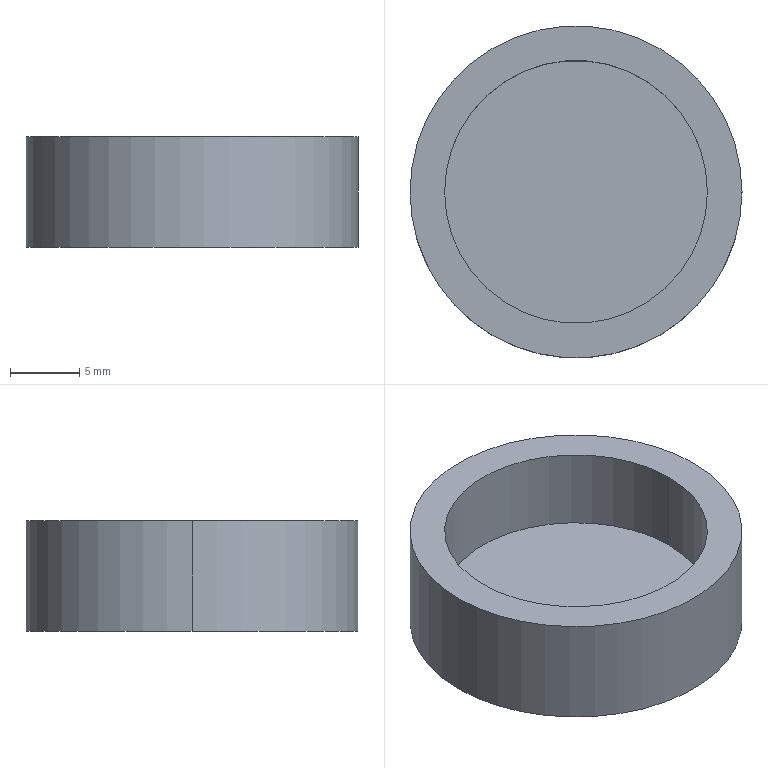Part | SolidWorks | features Extrusion 1, ICE 1 | 1 solid | 7 faces | box 24 x 24 x 8 mm | volume 1918 mm3 | cylinder 4 | plane 3 | commonest cylinder face diameters 19 x2 24 x2
STEP:
#1=CARTESIAN_POINT('',(-9.5,0.,2.));
#2=VERTEX_POINT('',#1);
#3=CARTESIAN_POINT('',(9.5,0.,2.));
#4=VERTEX_POINT('',#3);
#5=CARTESIAN_POINT('',(0.,0.,2.));
#6=DIRECTION('',(0.,0.,1.));
#7=DIRECTION('',(1.,0.,0.));
#8=AXIS2_PLACEMENT_3D('',#5,#6,#7);
#9=CIRCLE('',#8,9.5);
#10=EDGE_CURVE('',#2,#4,#9,.T.);
#11=ORIENTED_EDGE('',*,*,#10,.F.);
#12=CARTESIAN_POINT('',(-9.5,0.,8.));
#13=VERTEX_POINT('',#12);
#14=CARTESIAN_POINT('',(-9.5,0.,2.));
#15=DIRECTION('',(0.,0.,1.));
#16=VECTOR('',#15,1000.);
#17=LINE('',#14,#16);
#18=EDGE_CURVE('',#2,#13,#17,.T.);
#19=ORIENTED_EDGE('',*,*,#18,.T.);
#20=CARTESIAN_POINT('',(9.5,0.,8.));
#21=VERTEX_POINT('',#20);
#22=CARTESIAN_POINT('',(0.,0.,8.));
#23=DIRECTION('',(0.,0.,1.));
#24=DIRECTION('',(1.,0.,0.));
#25=AXIS2_PLACEMENT_3D('',#22,#23,#24);
#26=CIRCLE('',#25,9.5);
#27=EDGE_CURVE('',#13,#21,#26,.T.);
#28=ORIENTED_EDGE('',*,*,#27,.T.);
#29=CARTESIAN_POINT('',(9.5,0.,2.));
#30=DIRECTION('',(0.,0.,1.));
#31=VECTOR('',#30,1000.);
#32=LINE('',#29,#31);
#33=EDGE_CURVE('',#4,#21,#32,.T.);
#34=ORIENTED_EDGE('',*,*,#33,.F.);
#35=EDGE_LOOP('',(#11,#19,#28,#34));
#36=FACE_OUTER_BOUND('',#35,.T.);
#37=CARTESIAN_POINT('',(0.,0.,2.));
#38=DIRECTION('',(0.,0.,1.));
#39=DIRECTION('',(1.,0.,0.));
#40=AXIS2_PLACEMENT_3D('',#37,#38,#39);
#41=CYLINDRICAL_SURFACE('',#40,9.5);
#42=ADVANCED_FACE('',(#36),#41,.F.);
#43=CARTESIAN_POINT('',(12.,0.,8.));
#44=VERTEX_POINT('',#43);
#45=CARTESIAN_POINT('',(-12.,0.,8.));
#46=VERTEX_POINT('',#45);
#47=CARTESIAN_POINT('',(0.,0.,8.));
#48=DIRECTION('',(0.,0.,1.));
#49=DIRECTION('',(1.,0.,0.));
#50=AXIS2_PLACEMENT_3D('',#47,#48,#49);
#51=CIRCLE('',#50,12.);
#52=EDGE_CURVE('',#44,#46,#51,.T.);
#53=ORIENTED_EDGE('',*,*,#52,.F.);
#54=CARTESIAN_POINT('',(12.,0.,0.));
#55=VERTEX_POINT('',#54);
#56=CARTESIAN_POINT('',(12.,0.,8.));
#57=DIRECTION('',(0.,0.,-1.));
#58=VECTOR('',#57,1000.);
#59=LINE('',#56,#58);
#60=EDGE_CURVE('',#44,#55,#59,.T.);
#61=ORIENTED_EDGE('',*,*,#60,.T.);
#62=CARTESIAN_POINT('',(-12.,0.,0.));
#63=VERTEX_POINT('',#62);
#64=CARTESIAN_POINT('',(0.,0.,0.));
#65=DIRECTION('',(0.,0.,1.));
#66=DIRECTION('',(1.,0.,0.));
#67=AXIS2_PLACEMENT_3D('',#64,#65,#66);
#68=CIRCLE('',#67,12.);
#69=EDGE_CURVE('',#55,#63,#68,.T.);
#70=ORIENTED_EDGE('',*,*,#69,.T.);
#71=CARTESIAN_POINT('',(-12.,0.,8.));
#72=DIRECTION('',(0.,0.,-1.));
#73=VECTOR('',#72,1000.);
#74=LINE('',#71,#73);
#75=EDGE_CURVE('',#46,#63,#74,.T.);
#76=ORIENTED_EDGE('',*,*,#75,.F.);
#77=EDGE_LOOP('',(#53,#61,#70,#76));
#78=FACE_OUTER_BOUND('',#77,.T.);
#79=CARTESIAN_POINT('',(0.,0.,8.));
#80=DIRECTION('',(0.,0.,-1.));
#81=DIRECTION('',(-1.,0.,0.));
#82=AXIS2_PLACEMENT_3D('',#79,#80,#81);
#83=CYLINDRICAL_SURFACE('',#82,12.);
#84=ADVANCED_FACE('',(#78),#83,.T.);
#85=ORIENTED_EDGE('',*,*,#60,.F.);
#86=CARTESIAN_POINT('',(0.,0.,8.));
#87=DIRECTION('',(0.,0.,1.));
#88=DIRECTION('',(1.,0.,0.));
#89=AXIS2_PLACEMENT_3D('',#86,#87,#88);
#90=CIRCLE('',#89,12.);
#91=EDGE_CURVE('',#46,#44,#90,.T.);
#92=ORIENTED_EDGE('',*,*,#91,.F.);
#93=ORIENTED_EDGE('',*,*,#75,.T.);
#94=CARTESIAN_POINT('',(0.,0.,0.));
#95=DIRECTION('',(0.,0.,1.));
#96=DIRECTION('',(1.,0.,0.));
#97=AXIS2_PLACEMENT_3D('',#94,#95,#96);
#98=CIRCLE('',#97,12.);
#99=EDGE_CURVE('',#63,#55,#98,.T.);
#100=ORIENTED_EDGE('',*,*,#99,.T.);
#101=EDGE_LOOP('',(#85,#92,#93,#100));
#102=FACE_OUTER_BOUND('',#101,.T.);
#103=CARTESIAN_POINT('',(0.,0.,8.));
#104=DIRECTION('',(0.,0.,-1.));
#105=DIRECTION('',(-1.,0.,0.));
#106=AXIS2_PLACEMENT_3D('',#103,#104,#105);
#107=CYLINDRICAL_SURFACE('',#106,12.);
#108=ADVANCED_FACE('',(#102),#107,.T.);
#109=CARTESIAN_POINT('',(0.,0.,8.));
#110=DIRECTION('',(0.,0.,1.));
#111=DIRECTION('',(1.,0.,0.));
#112=AXIS2_PLACEMENT_3D('',#109,#110,#111);
#113=CIRCLE('',#112,9.5);
#114=EDGE_CURVE('',#21,#13,#113,.T.);
#115=ORIENTED_EDGE('',*,*,#114,.F.);
#116=ORIENTED_EDGE('',*,*,#27,.F.);
#117=EDGE_LOOP('',(#115,#116));
#118=FACE_BOUND('',#117,.T.);
#119=ORIENTED_EDGE('',*,*,#91,.T.);
#120=ORIENTED_EDGE('',*,*,#52,.T.);
#121=EDGE_LOOP('',(#119,#120));
#122=FACE_OUTER_BOUND('',#121,.T.);
#123=CARTESIAN_POINT('',(0.,0.,8.));
#124=DIRECTION('',(0.,0.,1.));
#125=DIRECTION('',(1.,0.,0.));
#126=AXIS2_PLACEMENT_3D('',#123,#124,#125);
#127=PLANE('',#126);
#128=ADVANCED_FACE('',(#118,#122),#127,.T.);
#129=ORIENTED_EDGE('',*,*,#99,.F.);
#130=ORIENTED_EDGE('',*,*,#69,.F.);
#131=EDGE_LOOP('',(#129,#130));
#132=FACE_OUTER_BOUND('',#131,.T.);
#133=CARTESIAN_POINT('',(0.,0.,0.));
#134=DIRECTION('',(0.,0.,1.));
#135=DIRECTION('',(1.,0.,0.));
#136=AXIS2_PLACEMENT_3D('',#133,#134,#135);
#137=PLANE('',#136);
#138=ADVANCED_FACE('',(#132),#137,.F.);
#139=ORIENTED_EDGE('',*,*,#18,.F.);
#140=CARTESIAN_POINT('',(0.,0.,2.));
#141=DIRECTION('',(0.,0.,1.));
#142=DIRECTION('',(1.,0.,0.));
#143=AXIS2_PLACEMENT_3D('',#140,#141,#142);
#144=CIRCLE('',#143,9.5);
#145=EDGE_CURVE('',#4,#2,#144,.T.);
#146=ORIENTED_EDGE('',*,*,#145,.F.);
#147=ORIENTED_EDGE('',*,*,#33,.T.);
#148=ORIENTED_EDGE('',*,*,#114,.T.);
#149=EDGE_LOOP('',(#139,#146,#147,#148));
#150=FACE_OUTER_BOUND('',#149,.T.);
#151=CARTESIAN_POINT('',(0.,0.,2.));
#152=DIRECTION('',(0.,0.,1.));
#153=DIRECTION('',(1.,0.,0.));
#154=AXIS2_PLACEMENT_3D('',#151,#152,#153);
#155=CYLINDRICAL_SURFACE('',#154,9.5);
#156=ADVANCED_FACE('',(#150),#155,.F.);
#157=ORIENTED_EDGE('',*,*,#145,.T.);
#158=ORIENTED_EDGE('',*,*,#10,.T.);
#159=EDGE_LOOP('',(#157,#158));
#160=FACE_OUTER_BOUND('',#159,.T.);
#161=CARTESIAN_POINT('',(0.,0.,2.));
#162=DIRECTION('',(0.,0.,1.));
#163=DIRECTION('',(1.,0.,0.));
#164=AXIS2_PLACEMENT_3D('',#161,#162,#163);
#165=PLANE('',#164);
#166=ADVANCED_FACE('',(#160),#165,.T.);
#167=CLOSED_SHELL('',(#42,#84,#108,#128,#138,#156,#166));
#168=MANIFOLD_SOLID_BREP('',#167);
#169=CARTESIAN_POINT('',(0.,0.,0.));
#170=DIRECTION('',(0.,0.,1.));
#171=DIRECTION('',(1.,0.,0.));
#172=AXIS2_PLACEMENT_3D('',#169,#170,#171);
#173=(LENGTH_UNIT()NAMED_UNIT(*)SI_UNIT(.MILLI.,.METRE.));
#174=UNCERTAINTY_MEASURE_WITH_UNIT(LENGTH_MEASURE(0.00001),#173,'','');
#175=(NAMED_UNIT(*)PLANE_ANGLE_UNIT()SI_UNIT($,.RADIAN.));
#176=(NAMED_UNIT(*)SI_UNIT($,.STERADIAN.)SOLID_ANGLE_UNIT());
#177=(GEOMETRIC_REPRESENTATION_CONTEXT(3)GLOBAL_UNCERTAINTY_ASSIGNED_CONTEXT((#174))GLOBAL_UNIT_ASSIGNED_CONTEXT((#173,#175,#176))REPRESENTATION_CONTEXT('',''));
#178=ADVANCED_BREP_SHAPE_REPRESENTATION('',(#168,#172),#177);